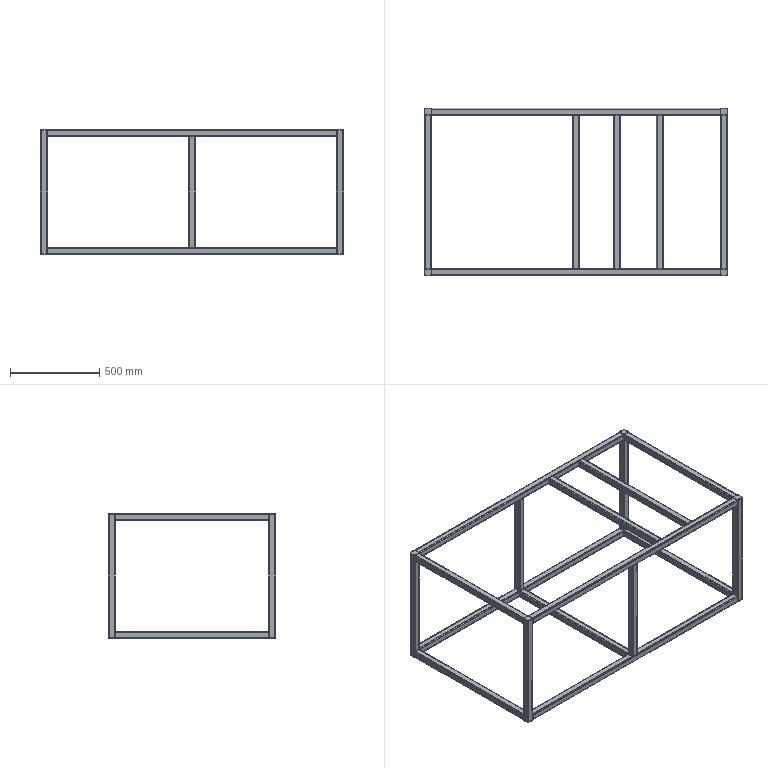Part | STEP file | 001-001-Profile frame_default<machined> | 25 solids | 386 faces | box 1700 x 940 x 700 mm | volume 7004652 mm3 | plane 250 | cylinder 136 | commonest cylinder face diameters 6 x68 12 x68